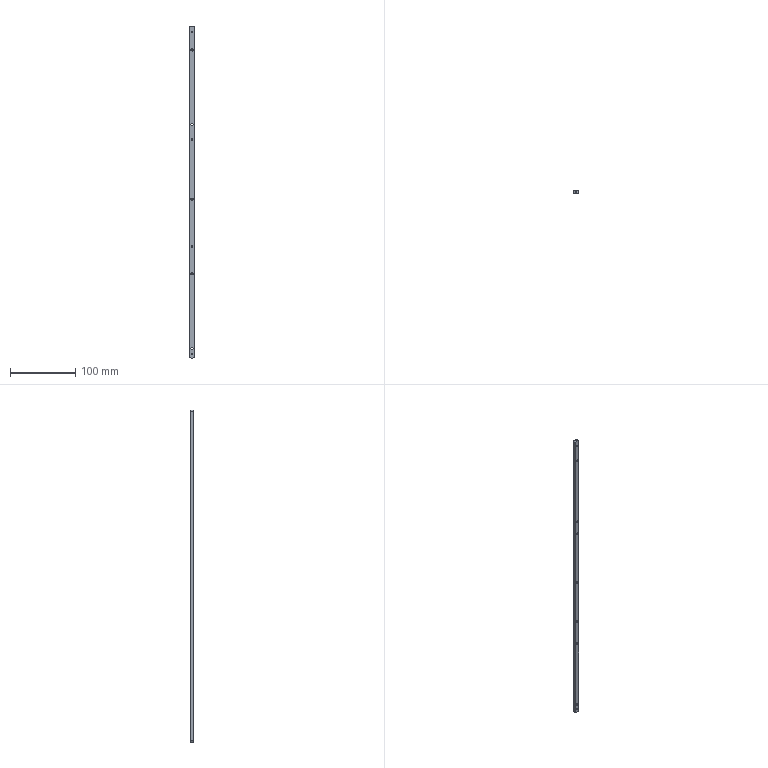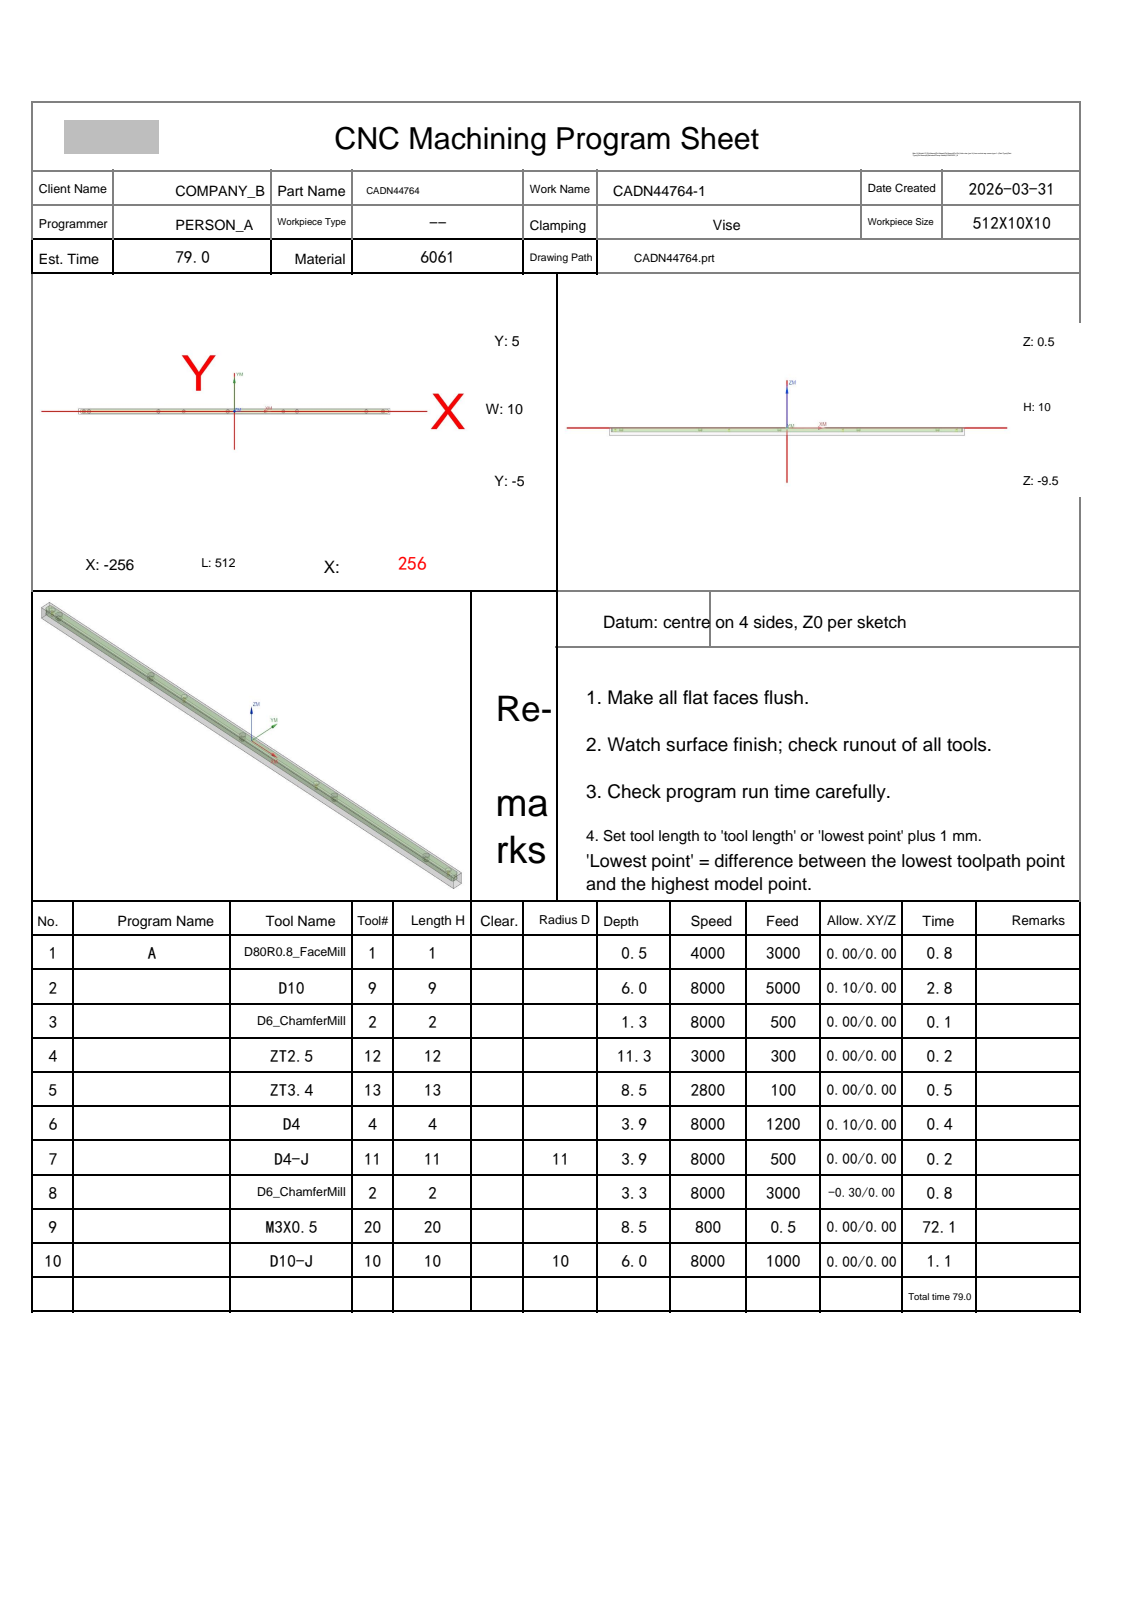NC program | NX | posted by the shop | part box 7 x 5 x 507 mm
Whole program:
%
O0001
(Machine time: 145.01 MIN)
(===Total Tool:9===)
(T1=D80R0.8 FaceMill D=80.  R=0.8  D-  H01 Z=0.    )
(T9=D10     D=10.  R=0.   D-  H09 Z=-5.5  )
(T2=D6_ChamferMill   D=6.   R=0.   D-  H02 Z=-2.75 )
(T12=ZT2.5  D=2.5  DR_a=118 D-  H12 Z=-10.75)
(T13=ZT3.4  D=3.4  DR_a=118 D-  H13 Z=-8.02 )
(T4=D4      D=4.   R=0.   D-  H04 Z=-3.4  )
(T11=D4-J   D=4.   R=0.   D11 H11 Z=-3.4  )
(T20=M3X0.5 D=2.5  DR_a=180 D-  H20 Z=-8.   )
(T10=D10-J  D=10.  R=0.   D10 H10 Z=-5.5  )
G80 G90 G17 G49 G40
G91 G28 Z0
M01
N1 T01 M06
(D80R0.8 FaceMill  D=80. R=0.8 H=01 ce=0.20 di=0.10)
G00 G90 G54 X298.5 Y0.0 M03 S4000
G43 H01 Z20.
M08
Z2.1
G01 Z.1 F3000.
X293.5
X-293.5
X-298.5
Z2.1
G00 Z20.
G00 G90 X298.5 Y0.0 M03 S4000
Z20.
Z2.
G01 Z0.0 F1000.
X293.5
X-293.5
X-298.5
Z2.
G00 Z20.
G91 G28 Z0.0
M05
M09
G91 G28 Z0.0
M01
N2 T09 M06
(D10  D=10. R=0. H=09 ce=0.10 di=0.00)
G00 G90 G54 X0.0 Y8.6 M03 S8000
G43 H09 Z20.
M08
Z.5
G01 X251.5 Z.381 F5000.
G02 X258.6 Y1.5 Z.376 I0.0 J-7.1
G01 Y-1.5 Z.374
G02 X251.5 Y-8.6 Z.369 I-7.1 J0.0
G01 X-251.5 Z.131
G02 X-258.6 Y-1.5 Z.126 I0.0 J7.1
G01 Y1.5 Z.124
G02 X-251.5 Y8.6 Z.119 I7.1 J0.0
G01 X251.5 Z-.119
G02 X258.6 Y1.5 Z-.124 I0.0 J-7.1
G01 Y-1.5 Z-.126
G02 X251.5 Y-8.6 Z-.131 I-7.1 J0.0
G01 X-251.5 Z-.369
G02 X-258.6 Y-1.5 Z-.374 I0.0 J7.1
G01 Y1.5 Z-.376
G02 X-251.5 Y8.6 Z-.381 I7.1 J0.0
G01 X251.5 Z-.619
G02 X258.6 Y1.5 Z-.624 I0.0 J-7.1
G01 Y-1.5 Z-.626
G02 X251.5 Y-8.6 Z-.631 I-7.1 J0.0
G01 X-251.5 Z-.869
G02 X-258.6 Y-1.5 Z-.874 I0.0 J7.1
G01 Y1.5 Z-.876
G02 X-251.5 Y8.6 Z-.881 I7.1 J0.0
G01 X251.5 Z-1.119
G02 X258.6 Y1.5 Z-1.124 I0.0 J-7.1
G01 Y-1.5 Z-1.126
G02 X251.5 Y-8.6 Z-1.131 I-7.1 J0.0
G01 X-251.5 Z-1.369
G02 X-258.6 Y-1.5 Z-1.374 I0.0 J7.1
G01 Y1.5 Z-1.376
G02 X-251.5 Y8.6 Z-1.381 I7.1 J0.0
G01 X251.5 Z-1.619
G02 X258.6 Y1.5 Z-1.624 I0.0 J-7.1
G01 Y-1.5 Z-1.626
G02 X251.5 Y-8.6 Z-1.631 I-7.1 J0.0
G01 X-251.5 Z-1.869
G02 X-258.6 Y-1.5 Z-1.874 I0.0 J7.1
G01 Y1.5 Z-1.876
G02 X-251.5 Y8.6 Z-1.881 I7.1 J0.0
G01 X251.5 Z-2.119
G02 X258.6 Y1.5 Z-2.124 I0.0 J-7.1
G01 Y-1.5 Z-2.126
G02 X251.5 Y-8.6 Z-2.131 I-7.1 J0.0
G01 X-251.5 Z-2.369
G02 X-258.6 Y-1.5 Z-2.374 I0.0 J7.1
G01 Y1.5 Z-2.376
G02 X-251.5 Y8.6 Z-2.381 I7.1 J0.0
G01 X251.5 Z-2.619
G02 X258.6 Y1.5 Z-2.624 I0.0 J-7.1
G01 Y-1.5 Z-2.626
G02 X251.5 Y-8.6 Z-2.631 I-7.1 J0.0
G01 X-251.5 Z-2.869
G02 X-258.6 Y-1.5 Z-2.874 I0.0 J7.1
G01 Y1.5 Z-2.876
G02 X-251.5 Y8.6 Z-2.881 I7.1 J0.0
G01 X251.5 Z-3.119
G02 X258.6 Y1.5 Z-3.124 I0.0 J-7.1
G01 Y-1.5 Z-3.126
G02 X251.5 Y-8.6 Z-3.131 I-7.1 J0.0
G01 X-251.5 Z-3.369
G02 X-258.6 Y-1.5 Z-3.374 I0.0 J7.1
G01 Y1.5 Z-3.376
G02 X-251.5 Y8.6 Z-3.381 I7.1 J0.0
G01 X251.5 Z-3.619
G02 X258.6 Y1.5 Z-3.624 I0.0 J-7.1
G01 Y-1.5 Z-3.626
G02 X251.5 Y-8.6 Z-3.631 I-7.1 J0.0
G01 X-251.5 Z-3.869
G02 X-258.6 Y-1.5 Z-3.874 I0.0 J7.1
G01 Y1.5 Z-3.876
G02 X-251.5 Y8.6 Z-3.881 I7.1 J0.0
G01 X251.5 Z-4.119
G02 X258.6 Y1.5 Z-4.124 I0.0 J-7.1
G01 Y-1.5 Z-4.126
G02 X251.5 Y-8.6 Z-4.131 I-7.1 J0.0
G01 X-251.5 Z-4.369
G02 X-258.6 Y-1.5 Z-4.374 I0.0 J7.1
G01 Y1.5 Z-4.376
G02 X-251.5 Y8.6 Z-4.381 I7.1 J0.0
G01 X251.5 Z-4.619
G02 X258.6 Y1.5 Z-4.624 I0.0 J-7.1
G01 Y-1.5 Z-4.626
G02 X251.5 Y-8.6 Z-4.631 I-7.1 J0.0
G01 X-251.5 Z-4.869
G02 X-258.6 Y-1.5 Z-4.874 I0.0 J7.1
G01 Y1.5 Z-4.876
G02 X-251.5 Y8.6 Z-4.881 I7.1 J0.0
G01 X251.5 Z-5.119
G02 X258.6 Y1.5 Z-5.124 I0.0 J-7.1
G01 Y-1.5 Z-5.126
G02 X251.5 Y-8.6 Z-5.131 I-7.1 J0.0
G01 X-251.5 Z-5.369
G02 X-258.6 Y-1.5 Z-5.374 I0.0 J7.1
G01 Y1.5 Z-5.376
G02 X-251.5 Y8.6 Z-5.381 I7.1 J0.0
G01 X0.0 Z-5.5
X251.5
G02 X258.6 Y1.5 I0.0 J-7.1
G01 Y-1.5
G02 X251.5 Y-8.6 I-7.1 J0.0
G01 X-251.5
G02 X-258.6 Y-1.5 I0.0 J7.1
G01 Y1.5
G02 X-251.5 Y8.6 I7.1 J0.0
G01 X0.0
X.5
Z-4.5
G00 Z20.
G91 G28 Z0.0
M05
M09
G91 G28 Z0.0
M01
N3 T02 M06
(D6_ChamferMill  D=6. R=0. H=02 ce=0.00 di=0.00)
G00 G90 G54 X-247.5 Y0.0 M03 S8000
G43 H02 Z20.
M08
G98 G81 X-247.5 Y0.0 Z-.8 R1. F500.
X-239.
X-125.
X-83.5
X-11.
X80.5
X103.
X217.
X244.5
G80
G00 Z20.
G91 G28 Z0.0
M05
M09
G91 G28 Z0.0
M01
N4 T12 M06
(ZT2.5 D=2.5 DR_a=118 H=12)
G00 G90 G54 X-247.5 Y0.0 M03 S3000
G43 H12 Z20.
M08
G98 G83 X-247.5 Y0.0 Z-10.751 R1. F300. Q2.
X-83.5
X80.5
X244.5
G80
G00 Z20.
G91 G28 Z0.0
M05
M09
G91 G28 Z0.0
M01
N5 T13 M06
(ZT3.4 D=3.4 DR_a=118 H=13)
G00 G90 G54 X-239. Y0.0 M03 S2800
G43 H13 Z20.
M08
G98 G83 X-239. Y0.0 Z-8.021 R1. F100. Q2.
X-125.
X-11.
X103.
X217.
G80
G00 Z20.
G91 G28 Z0.0
M05
M09
G91 G28 Z0.0
M01
N6 T04 M06
(D4  D=4. R=0. H=04 ce=0.10 di=0.00)
G00 G90 G54 X-239. Y0.0 M03 S8000
G43 H04 Z20.
M08
Z.5
G03 X-238.55 Y.45 I0.0 J.45 F1200.
X-239. Y.9 I-.45 J0.0
X-239. Y.9 Z.2 I0.0 J-.9
X-239. Y.9 Z-.1 I0.0 J-.9
X-239. Y.9 Z-.4 I0.0 J-.9
X-239. Y.9 Z-.7 I0.0 J-.9
X-239. Y.9 Z-1. I0.0 J-.9
X-239. Y.9 Z-1.3 I0.0 J-.9
X-239. Y.9 Z-1.6 I0.0 J-.9
X-239. Y.9 Z-1.9 I0.0 J-.9
X-239. Y.9 Z-2.2 I0.0 J-.9
X-239. Y.9 Z-2.5 I0.0 J-.9
X-239. Y.9 Z-2.8 I0.0 J-.9
X-239. Y.9 Z-3.1 I0.0 J-.9
X-239. Y.9 Z-3.4 I0.0 J-.9
X-239.9 Y0.0 I0.0 J-.9
X-239. Y-.9 I.9 J0.0
X-238.1 Y0.0 I0.0 J.9
X-239. Y.9 I-.9 J0.0
X-239.45 Y.45 I0.0 J-.45
X-239. Y0.0 I.45 J0.0
G00 Z20.
X-125.
Z.5
G03 X-124.55 Y.45 I0.0 J.45
X-125. Y.9 I-.45 J0.0
X-125. Y.9 Z.2 I0.0 J-.9
X-125. Y.9 Z-.1 I0.0 J-.9
X-125. Y.9 Z-.4 I0.0 J-.9
X-125. Y.9 Z-.7 I0.0 J-.9
X-125. Y.9 Z-1. I0.0 J-.9
X-125. Y.9 Z-1.3 I0.0 J-.9
X-125. Y.9 Z-1.6 I0.0 J-.9
X-125. Y.9 Z-1.9 I0.0 J-.9
X-125. Y.9 Z-2.2 I0.0 J-.9
X-125. Y.9 Z-2.5 I0.0 J-.9
X-125. Y.9 Z-2.8 I0.0 J-.9
X-125. Y.9 Z-3.1 I0.0 J-.9
X-125. Y.9 Z-3.4 I0.0 J-.9
X-125.9 Y0.0 I0.0 J-.9
X-125. Y-.9 I.9 J0.0
X-124.1 Y0.0 I0.0 J.9
X-125. Y.9 I-.9 J0.0
X-125.45 Y.45 I0.0 J-.45
X-125. Y0.0 I.45 J0.0
G00 Z20.
X-11.
Z.5
G03 X-10.55 Y.45 I0.0 J.45
X-11. Y.9 I-.45 J0.0
X-11. Y.9 Z.2 I0.0 J-.9
X-11. Y.9 Z-.1 I0.0 J-.9
X-11. Y.9 Z-.4 I0.0 J-.9
X-11. Y.9 Z-.7 I0.0 J-.9
X-11. Y.9 Z-1. I0.0 J-.9
X-11. Y.9 Z-1.3 I0.0 J-.9
X-11. Y.9 Z-1.6 I0.0 J-.9
X-11. Y.9 Z-1.9 I0.0 J-.9
X-11. Y.9 Z-2.2 I0.0 J-.9
X-11. Y.9 Z-2.5 I0.0 J-.9
X-11. Y.9 Z-2.8 I0.0 J-.9
X-11. Y.9 Z-3.1 I0.0 J-.9
X-11. Y.9 Z-3.4 I0.0 J-.9
X-11.9 Y0.0 I0.0 J-.9
X-11. Y-.9 I.9 J0.0
X-10.1 Y0.0 I0.0 J.9
X-11. Y.9 I-.9 J0.0
X-11.45 Y.45 I0.0 J-.45
X-11. Y0.0 I.45 J0.0
G00 Z20.
X103.
Z.5
G03 X103.45 Y.45 I0.0 J.45
X103. Y.9 I-.45 J0.0
X103. Y.9 Z.2 I0.0 J-.9
X103. Y.9 Z-.1 I0.0 J-.9
X103. Y.9 Z-.4 I0.0 J-.9
X103. Y.9 Z-.7 I0.0 J-.9
X103. Y.9 Z-1. I0.0 J-.9
X103. Y.9 Z-1.3 I0.0 J-.9
X103. Y.9 Z-1.6 I0.0 J-.9
X103. Y.9 Z-1.9 I0.0 J-.9
X103. Y.9 Z-2.2 I0.0 J-.9
X103. Y.9 Z-2.5 I0.0 J-.9
X103. Y.9 Z-2.8 I0.0 J-.9
X103. Y.9 Z-3.1 I0.0 J-.9
X103. Y.9 Z-3.4 I0.0 J-.9
X102.1 Y0.0 I0.0 J-.9
X103. Y-.9 I.9 J0.0
X103.9 Y0.0 I0.0 J.9
X103. Y.9 I-.9 J0.0
X102.55 Y.45 I0.0 J-.45
X103. Y0.0 I.45 J0.0
G00 Z20.
X217.
Z.5
G03 X217.45 Y.45 I0.0 J.45
X217. Y.9 I-.45 J0.0
X217. Y.9 Z.2 I0.0 J-.9
X217. Y.9 Z-.1 I0.0 J-.9
X217. Y.9 Z-.4 I0.0 J-.9
X217. Y.9 Z-.7 I0.0 J-.9
X217. Y.9 Z-1. I0.0 J-.9
X217. Y.9 Z-1.3 I0.0 J-.9
X217. Y.9 Z-1.6 I0.0 J-.9
X217. Y.9 Z-1.9 I0.0 J-.9
X217. Y.9 Z-2.2 I0.0 J-.9
X217. Y.9 Z-2.5 I0.0 J-.9
X217. Y.9 Z-2.8 I0.0 J-.9
X217. Y.9 Z-3.1 I0.0 J-.9
X217. Y.9 Z-3.4 I0.0 J-.9
X216.1 Y0.0 I0.0 J-.9
X217. Y-.9 I.9 J0.0
X217.9 Y0.0 I0.0 J.9
X217. Y.9 I-.9 J0.0
X216.55 Y.45 I0.0 J-.45
X217. Y0.0 I.45 J0.0
G00 Z20.
G91 G28 Z0.0
M05
M09
G91 G28 Z0.0
M01
N7 T11 M06
(D4-J  D=4. R=0. H=11 ce=0.00 di=0.00)
G00 G90 G54 X-239. Y0.0 M03 S8000
G43 H11 Z20.
M08
Z.5
G41 D11
G01 X-238.815 Y.077 F500.
G03 X-238.52 Y.52 I-.185 J.443
X-239. Y1. I-.48 J0.0
X-238.018 Y.187 Z-3.4 I0.0 J-1.
X-239. Y1. I-.982 J-.187
X-240. Y0.0 I0.0 J-1.
X-239. Y-1. I1. J0.0
X-238. Y0.0 I0.0 J1.
G01 X-238.018 Y.187
G03 X-238.489 Y.577 I-.471 J-.09
X-238.959 Y.196 I0.0 J-.48
G01 G40 X-239. Y0.0
G00 Z20.
X-125.
Z.5
G41 D11
G01 X-124.815 Y.077
G03 X-124.52 Y.52 I-.185 J.443
X-125. Y1. I-.48 J0.0
X-124.018 Y.187 Z-3.4 I0.0 J-1.
X-125. Y1. I-.982 J-.187
X-126. Y0.0 I0.0 J-1.
X-125. Y-1. I1. J0.0
X-124. Y0.0 I0.0 J1.
G01 X-124.018 Y.187
G03 X-124.489 Y.577 I-.471 J-.09
X-124.959 Y.196 I0.0 J-.48
G01 G40 X-125. Y0.0
G00 Z20.
X-11.
Z.5
G41 D11
G01 X-10.815 Y.077
G03 X-10.52 Y.52 I-.185 J.443
X-11. Y1. I-.48 J0.0
X-10.018 Y.187 Z-3.4 I0.0 J-1.
X-11. Y1. I-.982 J-.187
X-12. Y0.0 I0.0 J-1.
X-11. Y-1. I1. J0.0
X-10. Y0.0 I0.0 J1.
G01 X-10.018 Y.187
G03 X-10.489 Y.577 I-.471 J-.09
X-10.959 Y.196 I0.0 J-.48
G01 G40 X-11. Y0.0
G00 Z20.
X103.
Z.5
G41 D11
G01 X103.185 Y.077
G03 X103.48 Y.52 I-.185 J.443
X103. Y1. I-.48 J0.0
X103.982 Y.187 Z-3.4 I0.0 J-1.
X103. Y1. I-.982 J-.187
X102. Y0.0 I0.0 J-1.
X103. Y-1. I1. J0.0
X104. Y0.0 I0.0 J1.
G01 X103.982 Y.187
G03 X103.511 Y.577 I-.471 J-.09
X103.041 Y.196 I0.0 J-.48
G01 G40 X103. Y0.0
G00 Z20.
X217.
Z.5
G41 D11
G01 X217.185 Y.077
G03 X217.48 Y.52 I-.185 J.443
X217. Y1. I-.48 J0.0
X217.982 Y.187 Z-3.4 I0.0 J-1.
X217. Y1. I-.982 J-.187
X216. Y0.0 I0.0 J-1.
X217. Y-1. I1. J0.0
X218. Y0.0 I0.0 J1.
G01 X217.982 Y.187
G03 X217.511 Y.577 I-.471 J-.09
X217.041 Y.196 I0.0 J-.48
G01 G40 X217. Y0.0
G00 Z20.
G91 G28 Z0.0
M05
M09
G91 G28 Z0.0
M01
N8 T02 M06
(D6_ChamferMill  D=6. R=0. H=02 ce=0.00 di=0.00)
G00 G90 G54 X.25 Y-5.628 M03 S8000
G43 H02 Z20.
M08
Z2.099
G01 Z-1.5 F3000.
G03 X.33 Y-5.328 I-.52 J.3
X.03 Y-4.808 I-.6 J0.0
G01 X0.0 Y-4.8
X-251.5
G02 X-254.8 Y-1.5 I0.0 J3.3
G01 Y1.5
G02 X-251.5 Y4.8 I3.3 J0.0
G01 X251.5
G02 X254.8 Y1.5 I0.0 J-3.3
G01 Y-1.5
G02 X251.5 Y-4.8 I-3.3 J0.0
G01 X0.0
X-.03 Y-4.808
G03 X-.33 Y-5.328 I.3 J-.52
X-.25 Y-5.628 I.6 J0.0
G01 Z2.099
G00 Z20.
G00 G90 X-247.5 Y0.0 M03 S8000
Z20.
G98 G81 X-247.5 Y0.0 Z-2.75 R3. F500.
X-83.5
X80.5
X244.5
G80
G00 Z20.
G00 G90 X218.17 Y-1.981 M03 S8000
Z20.
Z2.5
G01 X218.252 Y-1.933 Z2.465 F500.
X218.513 Y-1.736 Z2.346
X218.744 Y-1.504 Z2.227
X218.94 Y-1.241 Z2.108
X219.096 Y-.954 Z1.989
X219.21 Y-.647 Z1.87
X219.28 Y-.327 Z1.75
X219.303 Y0.0 Z1.631
X219.28 Y.327 Z1.512
X219.21 Y.647 Z1.393
X219.096 Y.954 Z1.274
X218.94 Y1.241 Z1.154
X218.744 Y1.504 Z1.035
X218.513 Y1.736 Z.916
X218.252 Y1.933 Z.797
X218.048 Y2.051 Z.711
X217.747 Y2.179 Z.592
X217.43 Y2.262 Z.473
X217.105 Y2.301 Z.354
X216.778 Y2.292 Z.235
X216.455 Y2.238 Z.115
X216.143 Y2.138 Z-.004
X215.849 Y1.994 Z-.123
X215.577 Y1.811 Z-.242
X215.335 Y1.591 Z-.361
X215.126 Y1.339 Z-.48
X214.955 Y1.059 Z-.6
X214.826 Y.759 Z-.719
X214.74 Y.443 Z-.838
X214.7 Y.118 Z-.957
Y0.0 Z-1.
G03 X217. Y-2.3 I2.3 J0.0
X219.3 Y0.0 I0.0 J2.3
X217. Y2.3 I-2.3 J0.0
X214.7 Y0.0 I0.0 J-2.3
X214.754 Y-.496 I2.3 J0.0
G01 Z1.5
G00 Z20.
X104.17 Y-1.981
Z2.5
G01 X104.252 Y-1.933 Z2.465
X104.513 Y-1.736 Z2.346
X104.744 Y-1.504 Z2.227
X104.94 Y-1.241 Z2.108
X105.096 Y-.954 Z1.989
X105.21 Y-.647 Z1.87
X105.28 Y-.327 Z1.75
X105.303 Y0.0 Z1.631
X105.28 Y.327 Z1.512
X105.21 Y.647 Z1.393
X105.096 Y.954 Z1.274
X104.94 Y1.241 Z1.154
X104.744 Y1.504 Z1.035
X104.513 Y1.736 Z.916
X104.252 Y1.933 Z.797
X104.048 Y2.051 Z.711
X103.747 Y2.179 Z.592
X103.43 Y2.262 Z.473
X103.105 Y2.301 Z.354
X102.778 Y2.292 Z.235
X102.455 Y2.238 Z.115
X102.143 Y2.138 Z-.004
X101.849 Y1.994 Z-.123
X101.577 Y1.811 Z-.242
X101.335 Y1.591 Z-.361
X101.126 Y1.339 Z-.48
X100.955 Y1.059 Z-.6
X100.826 Y.759 Z-.719
X100.74 Y.443 Z-.838
X100.7 Y.118 Z-.957
Y0.0 Z-1.
G03 X103. Y-2.3 I2.3 J0.0
X105.3 Y0.0 I0.0 J2.3
X103. Y2.3 I-2.3 J0.0
X100.7 Y0.0 I0.0 J-2.3
X100.754 Y-.496 I2.3 J0.0
G01 Z1.5
G00 Z20.
X-9.83 Y-1.981
Z2.5
G01 X-9.748 Y-1.933 Z2.465
X-9.487 Y-1.736 Z2.346
X-9.256 Y-1.504 Z2.227
X-9.06 Y-1.241 Z2.108
X-8.904 Y-.954 Z1.989
X-8.79 Y-.647 Z1.87
X-8.72 Y-.327 Z1.75
X-8.697 Y0.0 Z1.631
X-8.72 Y.327 Z1.512
X-8.79 Y.647 Z1.393
X-8.904 Y.954 Z1.274
X-9.06 Y1.241 Z1.154
X-9.256 Y1.504 Z1.035
X-9.487 Y1.736 Z.916
X-9.748 Y1.933 Z.797
X-9.952 Y2.051 Z.711
X-10.253 Y2.179 Z.592
X-10.57 Y2.262 Z.473
X-10.895 Y2.301 Z.354
X-11.222 Y2.292 Z.235
X-11.545 Y2.238 Z.115
X-11.857 Y2.138 Z-.004
X-12.152 Y1.994 Z-.123
X-12.423 Y1.811 Z-.242
X-12.665 Y1.591 Z-.361
X-12.874 Y1.339 Z-.48
X-13.045 Y1.059 Z-.6
X-13.174 Y.759 Z-.719
X-13.26 Y.443 Z-.838
X-13.3 Y.118 Z-.957
Y0.0 Z-1.
G03 X-11. Y-2.3 I2.3 J0.0
X-8.7 Y0.0 I0.0 J2.3
X-11. Y2.3 I-2.3 J0.0
X-13.3 Y0.0 I0.0 J-2.3
X-13.246 Y-.496 I2.3 J0.0
G01 Z1.5
G00 Z20.
X-123.83 Y-1.981
Z2.5
G01 X-123.748 Y-1.933 Z2.465
X-123.487 Y-1.736 Z2.346
X-123.256 Y-1.504 Z2.227
X-123.06 Y-1.241 Z2.108
X-122.904 Y-.954 Z1.989
X-122.79 Y-.647 Z1.87
X-122.72 Y-.327 Z1.75
X-122.697 Y0.0 Z1.631
X-122.72 Y.327 Z1.512
X-122.79 Y.647 Z1.393
X-122.904 Y.954 Z1.274
X-123.06 Y1.241 Z1.154
X-123.256 Y1.504 Z1.035
X-123.487 Y1.736 Z.916
X-123.748 Y1.933 Z.797
X-123.952 Y2.051 Z.711
X-124.253 Y2.179 Z.592
X-124.57 Y2.262 Z.473
X-124.895 Y2.301 Z.354
X-125.222 Y2.292 Z.235
X-125.545 Y2.238 Z.115
X-125.857 Y2.138 Z-.004
X-126.152 Y1.994 Z-.123
X-126.423 Y1.811 Z-.242
X-126.665 Y1.591 Z-.361
X-126.874 Y1.339 Z-.48
X-127.045 Y1.059 Z-.6
X-127.174 Y.759 Z-.719
X-127.26 Y.443 Z-.838
X-127.3 Y.118 Z-.957
Y0.0 Z-1.
G03 X-125. Y-2.3 I2.3 J0.0
X-122.7 Y0.0 I0.0 J2.3
X-125. Y2.3 I-2.3 J0.0
X-127.3 Y0.0 I0.0 J-2.3
X-127.246 Y-.496 I2.3 J0.0
G01 Z1.5
G00 Z20.
X-237.83 Y-1.981
Z2.5
G01 X-237.748 Y-1.933 Z2.465
X-237.487 Y-1.736 Z2.346
X-237.256 Y-1.504 Z2.227
X-237.06 Y-1.241 Z2.108
X-236.904 Y-.954 Z1.989
X-236.79 Y-.647 Z1.87
X-236.72 Y-.327 Z1.75
X-236.697 Y0.0 Z1.631
X-236.72 Y.327 Z1.512
X-236.79 Y.647 Z1.393
X-236.904 Y.954 Z1.274
X-237.06 Y1.241 Z1.154
X-237.256 Y1.504 Z1.035
X-237.487 Y1.736 Z.916
X-237.748 Y1.933 Z.797
X-237.952 Y2.051 Z.711
X-238.253 Y2.179 Z.592
X-238.57 Y2.262 Z.473
X-238.895 Y2.301 Z.354
X-239.222 Y2.292 Z.235
X-239.545 Y2.238 Z.115
X-239.857 Y2.138 Z-.004
X-240.152 Y1.994 Z-.123
X-240.423 Y1.811 Z-.242
X-240.665 Y1.591 Z-.361
X-240.874 Y1.339 Z-.48
X-241.045 Y1.059 Z-.6
X-241.174 Y.759 Z-.719
X-241.26 Y.443 Z-.838
X-241.3 Y.118 Z-.957
Y0.0 Z-1.
G03 X-239. Y-2.3 I2.3 J0.0
X-236.7 Y0.0 I0.0 J2.3
X-239. Y2.3 I-2.3 J0.0
X-241.3 Y0.0 I0.0 J-2.3
X-241.246 Y-.496 I2.3 J0.0
G01 Z1.5
G00 Z20.
G91 G28 Z0.0
M05
M09
G91 G28 Z0.0
M01
N9 T20 M06
(M3X0.5 D=2.5 DR_a=180 H=20)
G00 G90 G54 X-247.5 Y0.0 M03 S800
G43 H20 Z20.
M08
G95
G98 G84 X-247.5 Y0.0 Z-8. R1. F.5 Q5.
X-83.5
X80.5
X244.5
G80
G94
G00 Z20.
G91 G28 Z0.0
M05
M09
G91 G28 Z0.0
M01
N10 T10 M06
(D10-J  D=10. R=0. H=10 ce=0.00 di=0.00)
G00 G90 G54 X-252.511 Y9.637 M03 S8000
G43 H10 Z20.
M08
Z-5.
G01 Z-5.5 F1000.
G41 D10
X-252.498 Y9.438
G03 X-251.5 Y8.5 I.998 J.063
G01 X251.5
G02 X258.5 Y1.5 I0.0 J-7.
G01 Y-1.5
G02 X251.5 Y-8.5 I-7. J0.0
G01 X-251.5
G02 X-258.5 Y-1.5 I0.0 J7.
G01 Y1.5
G02 X-251.5 Y8.5 I7. J0.0
G01 X-251.
G03 X-250. Y9.5 I0.0 J1.
G01 G40 Y9.7
Z-5.
G00 Z20.
M05
M09
G91 G28 Z0.0
G91 G28 Y0.0
M30
%